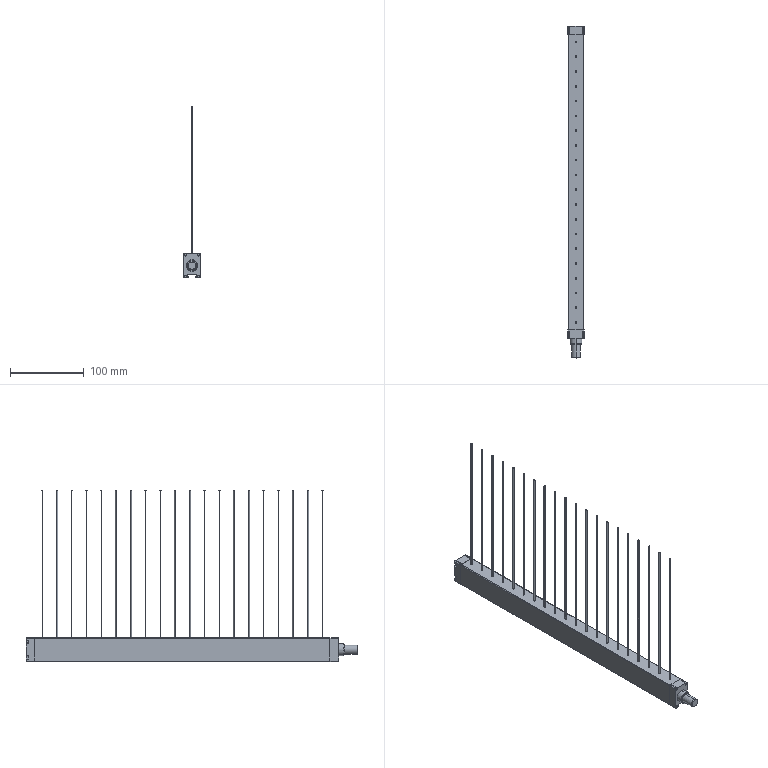Part | SolidWorks | features ICE 3, Extrusion 1, LPattern 1, MirrorPattern 1, Revolution 1 | 1 solid | 163 faces | box 22 x 450 x 232.8 mm | volume 289994 mm3 | plane 83 | cylinder 78 | cone 2 | commonest cylinder face diameters 2 x48 3 x16 1.6 x4 4 x4 12 x2 14 x2